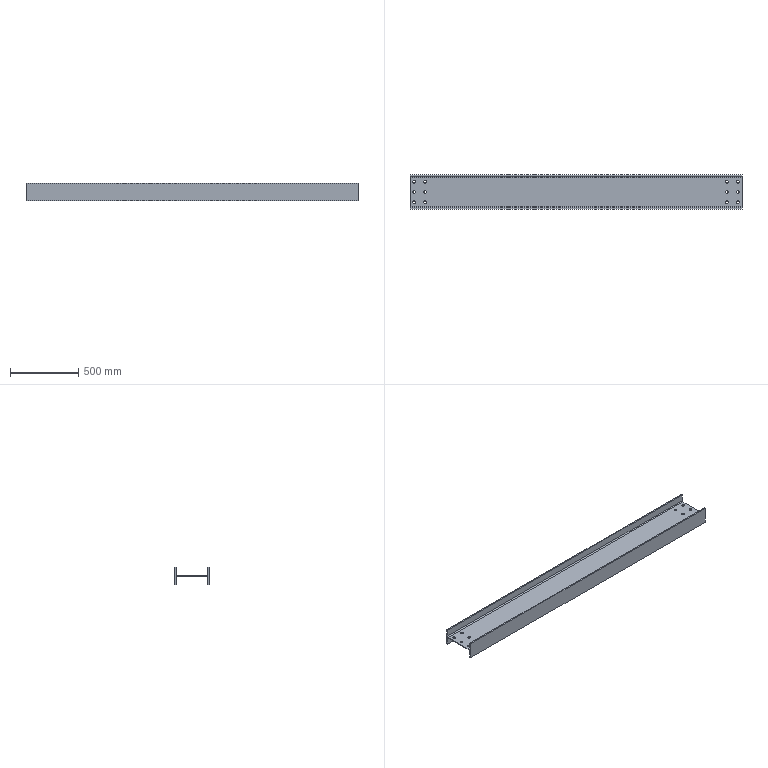Part | STEP file | 粉仓主梁3主体_Default<As Machined> | 1 solid | 42 faces | box 2430 x 250 x 125 mm | volume 8963145 mm3 | cylinder 28 | plane 14 | commonest cylinder face diameters 19 x24 16 x4